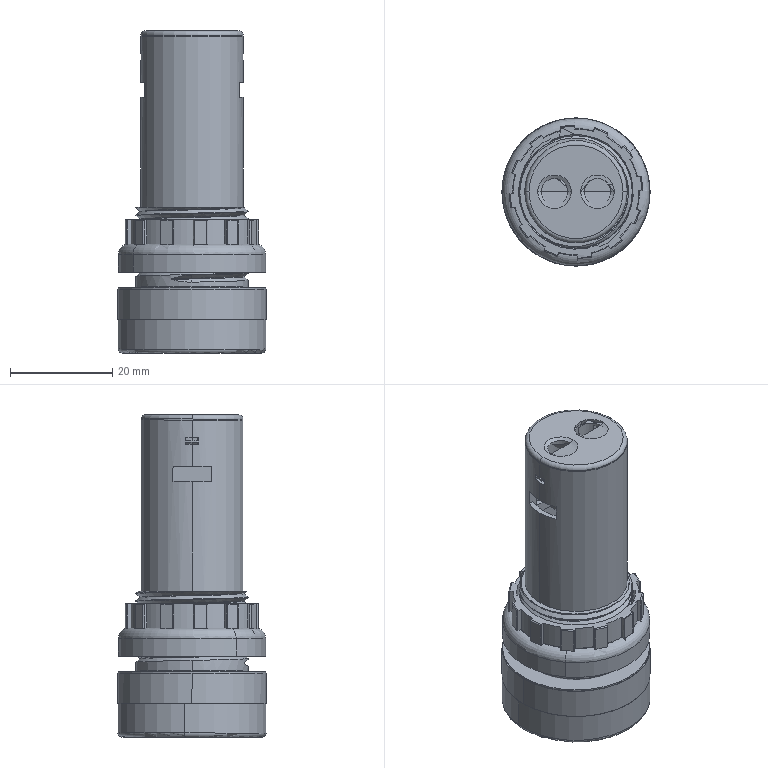Part | STEP file | indicator light AD17-22-AC220VW white | 3 solids | 410 faces | box 29 x 29.009 x 63.018 mm | volume 10026 mm3 | plane 192 | cylinder 170 | spline 31 | cone 9 | torus 8 | commonest cylinder face diameters 0.4 x40 22 x20 22.4 x18 24.6 x12 26.02 x11 1 x8